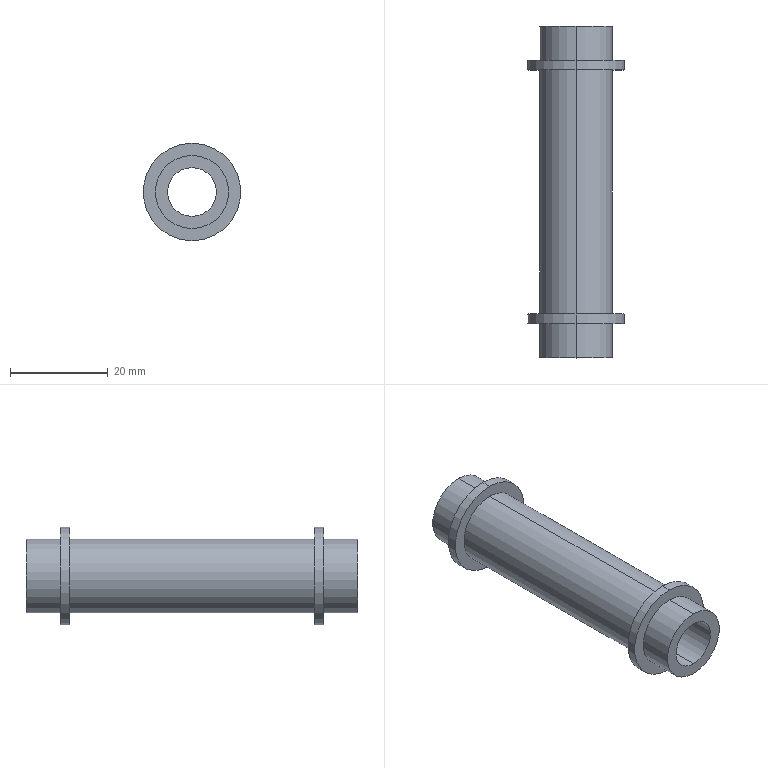Part | STEP file | 1 solid | 18 faces | box 20 x 68 x 20 mm | volume 7226 mm3 | cylinder 12 | plane 6 | commonest cylinder face diameters 15 x6 20 x4 10 x2
STEP:
#1=CARTESIAN_POINT('',(0.,0.,0.));
#2=DIRECTION('',(0.,0.,1.));
#3=DIRECTION('',(1.,0.,0.));
#4=AXIS2_PLACEMENT_3D('',#1,#2,#3);
#5=CARTESIAN_POINT('',(0.,9.,7.5));
#6=VERTEX_POINT('',#5);
#7=CARTESIAN_POINT('',(0.,9.,-7.5));
#8=VERTEX_POINT('',#7);
#9=CARTESIAN_POINT('',(0.,9.,0.));
#10=DIRECTION('',(0.,1.,0.));
#11=DIRECTION('',(0.,0.,1.));
#12=AXIS2_PLACEMENT_3D('',#9,#10,#11);
#13=CIRCLE('',#12,7.5);
#14=CARTESIAN_POINT('',(0.,0.,0.));
#15=DIRECTION('',(0.,1.,0.));
#16=DIRECTION('',(0.,0.,1.));
#17=AXIS2_PLACEMENT_3D('',#14,#15,#16);
#18=CYLINDRICAL_SURFACE('',#17,7.5);
#19=CARTESIAN_POINT('',(0.,9.));
#20=DIRECTION('',(1.,0.));
#21=VECTOR('',#20,1.);
#22=LINE('',#19,#21);
#23=(GEOMETRIC_REPRESENTATION_CONTEXT(2)PARAMETRIC_REPRESENTATION_CONTEXT()REPRESENTATION_CONTEXT('',''));
#24=DEFINITIONAL_REPRESENTATION('',(#22),#23);
#25=PCURVE('',#18,#24);
#26=CARTESIAN_POINT('',(0.,9.,0.));
#27=DIRECTION('',(0.,1.,0.));
#28=DIRECTION('',(0.,0.,1.));
#29=AXIS2_PLACEMENT_3D('',#26,#27,#28);
#30=PLANE('',#29);
#31=CARTESIAN_POINT('',(0.,0.));
#32=DIRECTION('',(1.,0.));
#33=AXIS2_PLACEMENT_2D('',#31,#32);
#34=CIRCLE('',#33,7.5);
#35=(GEOMETRIC_REPRESENTATION_CONTEXT(2)PARAMETRIC_REPRESENTATION_CONTEXT()REPRESENTATION_CONTEXT('',''));
#36=DEFINITIONAL_REPRESENTATION('',(#34),#35);
#37=PCURVE('',#30,#36);
#38=SURFACE_CURVE('',#13,(#25,#37),.PCURVE_S1.);
#39=EDGE_CURVE('',#6,#8,#38,.T.);
#40=ORIENTED_EDGE('',*,*,#39,.T.);
#41=CARTESIAN_POINT('',(0.,59.,-7.5));
#42=VERTEX_POINT('',#41);
#43=CARTESIAN_POINT('',(0.,0.,-7.5));
#44=DIRECTION('',(0.,1.,0.));
#45=VECTOR('',#44,1.);
#46=LINE('',#43,#45);
#47=CARTESIAN_POINT('',(3.142,0.));
#48=DIRECTION('',(0.,1.));
#49=VECTOR('',#48,1.);
#50=LINE('',#47,#49);
#51=(GEOMETRIC_REPRESENTATION_CONTEXT(2)PARAMETRIC_REPRESENTATION_CONTEXT()REPRESENTATION_CONTEXT('',''));
#52=DEFINITIONAL_REPRESENTATION('',(#50),#51);
#53=PCURVE('',#18,#52);
#54=CARTESIAN_POINT('',(0.,0.,0.));
#55=DIRECTION('',(0.,1.,0.));
#56=DIRECTION('',(0.,0.,1.));
#57=AXIS2_PLACEMENT_3D('',#54,#55,#56);
#58=CYLINDRICAL_SURFACE('',#57,7.5);
#59=CARTESIAN_POINT('',(3.142,0.));
#60=DIRECTION('',(0.,1.));
#61=VECTOR('',#60,1.);
#62=LINE('',#59,#61);
#63=(GEOMETRIC_REPRESENTATION_CONTEXT(2)PARAMETRIC_REPRESENTATION_CONTEXT()REPRESENTATION_CONTEXT('',''));
#64=DEFINITIONAL_REPRESENTATION('',(#62),#63);
#65=PCURVE('',#58,#64);
#66=SURFACE_CURVE('',#46,(#53,#65),.PCURVE_S1.);
#67=EDGE_CURVE('',#8,#42,#66,.T.);
#68=ORIENTED_EDGE('',*,*,#67,.T.);
#69=CARTESIAN_POINT('',(0.,59.,7.5));
#70=VERTEX_POINT('',#69);
#71=CARTESIAN_POINT('',(0.,59.,0.));
#72=DIRECTION('',(0.,-1.,0.));
#73=DIRECTION('',(0.,0.,1.));
#74=AXIS2_PLACEMENT_3D('',#71,#72,#73);
#75=CIRCLE('',#74,7.5);
#76=CARTESIAN_POINT('',(6.283,59.));
#77=DIRECTION('',(-1.,0.));
#78=VECTOR('',#77,1.);
#79=LINE('',#76,#78);
#80=(GEOMETRIC_REPRESENTATION_CONTEXT(2)PARAMETRIC_REPRESENTATION_CONTEXT()REPRESENTATION_CONTEXT('',''));
#81=DEFINITIONAL_REPRESENTATION('',(#79),#80);
#82=PCURVE('',#18,#81);
#83=CARTESIAN_POINT('',(0.,59.,0.));
#84=DIRECTION('',(0.,1.,0.));
#85=DIRECTION('',(0.,0.,1.));
#86=AXIS2_PLACEMENT_3D('',#83,#84,#85);
#87=PLANE('',#86);
#88=CARTESIAN_POINT('',(7.5,0.));
#89=CARTESIAN_POINT('',(7.5,-12.99));
#90=CARTESIAN_POINT('',(-3.75,-6.495));
#91=CARTESIAN_POINT('',(-15.,0.));
#92=CARTESIAN_POINT('',(-3.75,6.495));
#93=CARTESIAN_POINT('',(7.5,12.99));
#94=CARTESIAN_POINT('',(7.5,0.));
#95=(BOUNDED_CURVE()B_SPLINE_CURVE(2,(#88,#89,#90,#91,#92,#93,#94),.UNSPECIFIED.,.T.,.F.)B_SPLINE_CURVE_WITH_KNOTS((1,2,2,2,2,1),(-2.094,0.,2.094,4.189,6.283,8.378),.UNSPECIFIED.)CURVE()GEOMETRIC_REPRESENTATION_ITEM()RATIONAL_B_SPLINE_CURVE((1.,0.5,1.,0.5,1.,0.5,1.))REPRESENTATION_ITEM(''));
#96=(GEOMETRIC_REPRESENTATION_CONTEXT(2)PARAMETRIC_REPRESENTATION_CONTEXT()REPRESENTATION_CONTEXT('',''));
#97=DEFINITIONAL_REPRESENTATION('',(#95),#96);
#98=PCURVE('',#87,#97);
#99=SURFACE_CURVE('',#75,(#82,#98),.PCURVE_S1.);
#100=EDGE_CURVE('',#42,#70,#99,.T.);
#101=ORIENTED_EDGE('',*,*,#100,.T.);
#102=CARTESIAN_POINT('',(0.,0.,7.5));
#103=DIRECTION('',(0.,1.,0.));
#104=VECTOR('',#103,1.);
#105=LINE('',#102,#104);
#106=CARTESIAN_POINT('',(0.,0.));
#107=DIRECTION('',(0.,1.));
#108=VECTOR('',#107,1.);
#109=LINE('',#106,#108);
#110=(GEOMETRIC_REPRESENTATION_CONTEXT(2)PARAMETRIC_REPRESENTATION_CONTEXT()REPRESENTATION_CONTEXT('',''));
#111=DEFINITIONAL_REPRESENTATION('',(#109),#110);
#112=PCURVE('',#18,#111);
#113=CARTESIAN_POINT('',(6.283,0.));
#114=DIRECTION('',(0.,1.));
#115=VECTOR('',#114,1.);
#116=LINE('',#113,#115);
#117=(GEOMETRIC_REPRESENTATION_CONTEXT(2)PARAMETRIC_REPRESENTATION_CONTEXT()REPRESENTATION_CONTEXT('',''));
#118=DEFINITIONAL_REPRESENTATION('',(#116),#117);
#119=PCURVE('',#58,#118);
#120=SURFACE_CURVE('',#105,(#112,#119),.PCURVE_S1.);
#121=EDGE_CURVE('',#6,#70,#120,.T.);
#122=ORIENTED_EDGE('',*,*,#121,.F.);
#123=EDGE_LOOP('',(#40,#68,#101,#122));
#124=FACE_BOUND('',#123,.T.);
#125=ADVANCED_FACE('',(#124),#18,.T.);
#126=CARTESIAN_POINT('',(0.,9.,10.));
#127=VERTEX_POINT('',#126);
#128=CARTESIAN_POINT('',(0.,9.,-10.));
#129=VERTEX_POINT('',#128);
#130=CARTESIAN_POINT('',(0.,9.,0.));
#131=DIRECTION('',(0.,1.,0.));
#132=DIRECTION('',(0.,0.,-1.));
#133=AXIS2_PLACEMENT_3D('',#130,#131,#132);
#134=CIRCLE('',#133,10.);
#135=CARTESIAN_POINT('',(0.,9.,0.));
#136=DIRECTION('',(0.,-1.,0.));
#137=DIRECTION('',(0.,0.,-1.));
#138=AXIS2_PLACEMENT_3D('',#135,#136,#137);
#139=CYLINDRICAL_SURFACE('',#138,10.);
#140=CARTESIAN_POINT('',(6.283,0.));
#141=DIRECTION('',(-1.,0.));
#142=VECTOR('',#141,1.);
#143=LINE('',#140,#142);
#144=(GEOMETRIC_REPRESENTATION_CONTEXT(2)PARAMETRIC_REPRESENTATION_CONTEXT()REPRESENTATION_CONTEXT('',''));
#145=DEFINITIONAL_REPRESENTATION('',(#143),#144);
#146=PCURVE('',#139,#145);
#147=CARTESIAN_POINT('',(0.,0.));
#148=DIRECTION('',(-1.,0.));
#149=AXIS2_PLACEMENT_2D('',#147,#148);
#150=CIRCLE('',#149,10.);
#151=(GEOMETRIC_REPRESENTATION_CONTEXT(2)PARAMETRIC_REPRESENTATION_CONTEXT()REPRESENTATION_CONTEXT('',''));
#152=DEFINITIONAL_REPRESENTATION('',(#150),#151);
#153=PCURVE('',#30,#152);
#154=SURFACE_CURVE('',#134,(#146,#153),.PCURVE_S1.);
#155=EDGE_CURVE('',#127,#129,#154,.T.);
#156=ORIENTED_EDGE('',*,*,#155,.F.);
#157=CARTESIAN_POINT('',(0.,7.,10.));
#158=VERTEX_POINT('',#157);
#159=CARTESIAN_POINT('',(0.,9.,10.));
#160=DIRECTION('',(0.,-1.,0.));
#161=VECTOR('',#160,1.);
#162=LINE('',#159,#161);
#163=CARTESIAN_POINT('',(3.142,0.));
#164=DIRECTION('',(0.,1.));
#165=VECTOR('',#164,1.);
#166=LINE('',#163,#165);
#167=(GEOMETRIC_REPRESENTATION_CONTEXT(2)PARAMETRIC_REPRESENTATION_CONTEXT()REPRESENTATION_CONTEXT('',''));
#168=DEFINITIONAL_REPRESENTATION('',(#166),#167);
#169=PCURVE('',#139,#168);
#170=CARTESIAN_POINT('',(0.,9.,0.));
#171=DIRECTION('',(0.,-1.,0.));
#172=DIRECTION('',(0.,0.,-1.));
#173=AXIS2_PLACEMENT_3D('',#170,#171,#172);
#174=CYLINDRICAL_SURFACE('',#173,10.);
#175=CARTESIAN_POINT('',(3.142,0.));
#176=DIRECTION('',(0.,1.));
#177=VECTOR('',#176,1.);
#178=LINE('',#175,#177);
#179=(GEOMETRIC_REPRESENTATION_CONTEXT(2)PARAMETRIC_REPRESENTATION_CONTEXT()REPRESENTATION_CONTEXT('',''));
#180=DEFINITIONAL_REPRESENTATION('',(#178),#179);
#181=PCURVE('',#174,#180);
#182=SURFACE_CURVE('',#162,(#169,#181),.PCURVE_S1.);
#183=EDGE_CURVE('',#127,#158,#182,.T.);
#184=ORIENTED_EDGE('',*,*,#183,.T.);
#185=CARTESIAN_POINT('',(0.,7.,-10.));
#186=VERTEX_POINT('',#185);
#187=CARTESIAN_POINT('',(0.,7.,0.));
#188=DIRECTION('',(0.,1.,0.));
#189=DIRECTION('',(0.,0.,-1.));
#190=AXIS2_PLACEMENT_3D('',#187,#188,#189);
#191=CIRCLE('',#190,10.);
#192=CARTESIAN_POINT('',(6.283,2.));
#193=DIRECTION('',(-1.,0.));
#194=VECTOR('',#193,1.);
#195=LINE('',#192,#194);
#196=(GEOMETRIC_REPRESENTATION_CONTEXT(2)PARAMETRIC_REPRESENTATION_CONTEXT()REPRESENTATION_CONTEXT('',''));
#197=DEFINITIONAL_REPRESENTATION('',(#195),#196);
#198=PCURVE('',#139,#197);
#199=CARTESIAN_POINT('',(0.,7.,0.));
#200=DIRECTION('',(0.,1.,0.));
#201=DIRECTION('',(0.,0.,1.));
#202=AXIS2_PLACEMENT_3D('',#199,#200,#201);
#203=PLANE('',#202);
#204=CARTESIAN_POINT('',(0.,0.));
#205=DIRECTION('',(-1.,0.));
#206=AXIS2_PLACEMENT_2D('',#204,#205);
#207=CIRCLE('',#206,10.);
#208=(GEOMETRIC_REPRESENTATION_CONTEXT(2)PARAMETRIC_REPRESENTATION_CONTEXT()REPRESENTATION_CONTEXT('',''));
#209=DEFINITIONAL_REPRESENTATION('',(#207),#208);
#210=PCURVE('',#203,#209);
#211=SURFACE_CURVE('',#191,(#198,#210),.PCURVE_S1.);
#212=EDGE_CURVE('',#158,#186,#211,.T.);
#213=ORIENTED_EDGE('',*,*,#212,.T.);
#214=CARTESIAN_POINT('',(0.,9.,-10.));
#215=DIRECTION('',(0.,-1.,0.));
#216=VECTOR('',#215,1.);
#217=LINE('',#214,#216);
#218=CARTESIAN_POINT('',(0.,0.));
#219=DIRECTION('',(0.,1.));
#220=VECTOR('',#219,1.);
#221=LINE('',#218,#220);
#222=(GEOMETRIC_REPRESENTATION_CONTEXT(2)PARAMETRIC_REPRESENTATION_CONTEXT()REPRESENTATION_CONTEXT('',''));
#223=DEFINITIONAL_REPRESENTATION('',(#221),#222);
#224=PCURVE('',#139,#223);
#225=CARTESIAN_POINT('',(6.283,0.));
#226=DIRECTION('',(0.,1.));
#227=VECTOR('',#226,1.);
#228=LINE('',#225,#227);
#229=(GEOMETRIC_REPRESENTATION_CONTEXT(2)PARAMETRIC_REPRESENTATION_CONTEXT()REPRESENTATION_CONTEXT('',''));
#230=DEFINITIONAL_REPRESENTATION('',(#228),#229);
#231=PCURVE('',#174,#230);
#232=SURFACE_CURVE('',#217,(#224,#231),.PCURVE_S1.);
#233=EDGE_CURVE('',#129,#186,#232,.T.);
#234=ORIENTED_EDGE('',*,*,#233,.F.);
#235=EDGE_LOOP('',(#156,#184,#213,#234));
#236=FACE_BOUND('',#235,.T.);
#237=ADVANCED_FACE('',(#236),#139,.T.);
#238=CARTESIAN_POINT('',(0.,61.,-10.));
#239=VERTEX_POINT('',#238);
#240=CARTESIAN_POINT('',(0.,61.,10.));
#241=VERTEX_POINT('',#240);
#242=CARTESIAN_POINT('',(0.,61.,0.));
#243=DIRECTION('',(0.,-1.,0.));
#244=DIRECTION('',(0.,0.,-1.));
#245=AXIS2_PLACEMENT_3D('',#242,#243,#244);
#246=CIRCLE('',#245,10.);
#247=CARTESIAN_POINT('',(0.,59.,0.));
#248=DIRECTION('',(0.,-1.,0.));
#249=DIRECTION('',(0.,0.,-1.));
#250=AXIS2_PLACEMENT_3D('',#247,#248,#249);
#251=CYLINDRICAL_SURFACE('',#250,10.);
#252=CARTESIAN_POINT('',(0.,-2.));
#253=DIRECTION('',(1.,0.));
#254=VECTOR('',#253,1.);
#255=LINE('',#252,#254);
#256=(GEOMETRIC_REPRESENTATION_CONTEXT(2)PARAMETRIC_REPRESENTATION_CONTEXT()REPRESENTATION_CONTEXT('',''));
#257=DEFINITIONAL_REPRESENTATION('',(#255),#256);
#258=PCURVE('',#251,#257);
#259=CARTESIAN_POINT('',(0.,61.,0.));
#260=DIRECTION('',(0.,1.,0.));
#261=DIRECTION('',(0.,0.,1.));
#262=AXIS2_PLACEMENT_3D('',#259,#260,#261);
#263=PLANE('',#262);
#264=CARTESIAN_POINT('',(-10.,0.));
#265=CARTESIAN_POINT('',(-10.,17.321));
#266=CARTESIAN_POINT('',(5.,8.66));
#267=CARTESIAN_POINT('',(20.,0.));
#268=CARTESIAN_POINT('',(5.,-8.66));
#269=CARTESIAN_POINT('',(-10.,-17.321));
#270=CARTESIAN_POINT('',(-10.,0.));
#271=(BOUNDED_CURVE()B_SPLINE_CURVE(2,(#264,#265,#266,#267,#268,#269,#270),.UNSPECIFIED.,.T.,.F.)B_SPLINE_CURVE_WITH_KNOTS((1,2,2,2,2,1),(-2.094,0.,2.094,4.189,6.283,8.378),.UNSPECIFIED.)CURVE()GEOMETRIC_REPRESENTATION_ITEM()RATIONAL_B_SPLINE_CURVE((1.,0.5,1.,0.5,1.,0.5,1.))REPRESENTATION_ITEM(''));
#272=(GEOMETRIC_REPRESENTATION_CONTEXT(2)PARAMETRIC_REPRESENTATION_CONTEXT()REPRESENTATION_CONTEXT('',''));
#273=DEFINITIONAL_REPRESENTATION('',(#271),#272);
#274=PCURVE('',#263,#273);
#275=SURFACE_CURVE('',#246,(#258,#274),.PCURVE_S1.);
#276=EDGE_CURVE('',#239,#241,#275,.T.);
#277=ORIENTED_EDGE('',*,*,#276,.T.);
#278=CARTESIAN_POINT('',(0.,59.,10.));
#279=VERTEX_POINT('',#278);
#280=CARTESIAN_POINT('',(0.,59.,10.));
#281=DIRECTION('',(0.,-1.,0.));
#282=VECTOR('',#281,1.);
#283=LINE('',#280,#282);
#284=CARTESIAN_POINT('',(3.142,0.));
#285=DIRECTION('',(0.,1.));
#286=VECTOR('',#285,1.);
#287=LINE('',#284,#286);
#288=(GEOMETRIC_REPRESENTATION_CONTEXT(2)PARAMETRIC_REPRESENTATION_CONTEXT()REPRESENTATION_CONTEXT('',''));
#289=DEFINITIONAL_REPRESENTATION('',(#287),#288);
#290=PCURVE('',#251,#289);
#291=CARTESIAN_POINT('',(0.,59.,0.));
#292=DIRECTION('',(0.,-1.,0.));
#293=DIRECTION('',(0.,0.,-1.));
#294=AXIS2_PLACEMENT_3D('',#291,#292,#293);
#295=CYLINDRICAL_SURFACE('',#294,10.);
#296=CARTESIAN_POINT('',(3.142,0.));
#297=DIRECTION('',(0.,1.));
#298=VECTOR('',#297,1.);
#299=LINE('',#296,#298);
#300=(GEOMETRIC_REPRESENTATION_CONTEXT(2)PARAMETRIC_REPRESENTATION_CONTEXT()REPRESENTATION_CONTEXT('',''));
#301=DEFINITIONAL_REPRESENTATION('',(#299),#300);
#302=PCURVE('',#295,#301);
#303=SURFACE_CURVE('',#283,(#290,#302),.PCURVE_S1.);
#304=EDGE_CURVE('',#241,#279,#303,.T.);
#305=ORIENTED_EDGE('',*,*,#304,.T.);
#306=CARTESIAN_POINT('',(0.,59.,-10.));
#307=VERTEX_POINT('',#306);
#308=CARTESIAN_POINT('',(0.,59.,0.));
#309=DIRECTION('',(0.,1.,0.));
#310=DIRECTION('',(0.,0.,-1.));
#311=AXIS2_PLACEMENT_3D('',#308,#309,#310);
#312=CIRCLE('',#311,10.);
#313=CARTESIAN_POINT('',(6.283,0.));
#314=DIRECTION('',(-1.,0.));
#315=VECTOR('',#314,1.);
#316=LINE('',#313,#315);
#317=(GEOMETRIC_REPRESENTATION_CONTEXT(2)PARAMETRIC_REPRESENTATION_CONTEXT()REPRESENTATION_CONTEXT('',''));
#318=DEFINITIONAL_REPRESENTATION('',(#316),#317);
#319=PCURVE('',#251,#318);
#320=CARTESIAN_POINT('',(0.,0.));
#321=DIRECTION('',(-1.,0.));
#322=AXIS2_PLACEMENT_2D('',#320,#321);
#323=CIRCLE('',#322,10.);
#324=(GEOMETRIC_REPRESENTATION_CONTEXT(2)PARAMETRIC_REPRESENTATION_CONTEXT()REPRESENTATION_CONTEXT('',''));
#325=DEFINITIONAL_REPRESENTATION('',(#323),#324);
#326=PCURVE('',#87,#325);
#327=SURFACE_CURVE('',#312,(#319,#326),.PCURVE_S1.);
#328=EDGE_CURVE('',#279,#307,#327,.T.);
#329=ORIENTED_EDGE('',*,*,#328,.T.);
#330=CARTESIAN_POINT('',(0.,59.,-10.));
#331=DIRECTION('',(0.,-1.,0.));
#332=VECTOR('',#331,1.);
#333=LINE('',#330,#332);
#334=CARTESIAN_POINT('',(0.,0.));
#335=DIRECTION('',(0.,1.));
#336=VECTOR('',#335,1.);
#337=LINE('',#334,#336);
#338=(GEOMETRIC_REPRESENTATION_CONTEXT(2)PARAMETRIC_REPRESENTATION_CONTEXT()REPRESENTATION_CONTEXT('',''));
#339=DEFINITIONAL_REPRESENTATION('',(#337),#338);
#340=PCURVE('',#251,#339);
#341=CARTESIAN_POINT('',(6.283,0.));
#342=DIRECTION('',(0.,1.));
#343=VECTOR('',#342,1.);
#344=LINE('',#341,#343);
#345=(GEOMETRIC_REPRESENTATION_CONTEXT(2)PARAMETRIC_REPRESENTATION_CONTEXT()REPRESENTATION_CONTEXT('',''));
#346=DEFINITIONAL_REPRESENTATION('',(#344),#345);
#347=PCURVE('',#295,#346);
#348=SURFACE_CURVE('',#333,(#340,#347),.PCURVE_S1.);
#349=EDGE_CURVE('',#239,#307,#348,.T.);
#350=ORIENTED_EDGE('',*,*,#349,.F.);
#351=EDGE_LOOP('',(#277,#305,#329,#350));
#352=FACE_BOUND('',#351,.T.);
#353=ADVANCED_FACE('',(#352),#251,.T.);
#354=CARTESIAN_POINT('',(0.,0.,7.5));
#355=VERTEX_POINT('',#354);
#356=CARTESIAN_POINT('',(0.,0.,-7.5));
#357=VERTEX_POINT('',#356);
#358=CARTESIAN_POINT('',(0.,0.,0.));
#359=DIRECTION('',(0.,1.,0.));
#360=DIRECTION('',(0.,0.,1.));
#361=AXIS2_PLACEMENT_3D('',#358,#359,#360);
#362=CIRCLE('',#361,7.5);
#363=CARTESIAN_POINT('',(0.,0.,0.));
#364=DIRECTION('',(0.,1.,0.));
#365=DIRECTION('',(0.,0.,1.));
#366=AXIS2_PLACEMENT_3D('',#363,#364,#365);
#367=CYLINDRICAL_SURFACE('',#366,7.5);
#368=CARTESIAN_POINT('',(0.,0.));
#369=DIRECTION('',(1.,0.));
#370=VECTOR('',#369,1.);
#371=LINE('',#368,#370);
#372=(GEOMETRIC_REPRESENTATION_CONTEXT(2)PARAMETRIC_REPRESENTATION_CONTEXT()REPRESENTATION_CONTEXT('',''));
#373=DEFINITIONAL_REPRESENTATION('',(#371),#372);
#374=PCURVE('',#367,#373);
#375=CARTESIAN_POINT('',(0.,0.,0.));
#376=DIRECTION('',(0.,1.,0.));
#377=DIRECTION('',(0.,0.,1.));
#378=AXIS2_PLACEMENT_3D('',#375,#376,#377);
#379=PLANE('',#378);
#380=CARTESIAN_POINT('',(0.,0.));
#381=DIRECTION('',(1.,0.));
#382=AXIS2_PLACEMENT_2D('',#380,#381);
#383=CIRCLE('',#382,7.5);
#384=(GEOMETRIC_REPRESENTATION_CONTEXT(2)PARAMETRIC_REPRESENTATION_CONTEXT()REPRESENTATION_CONTEXT('',''));
#385=DEFINITIONAL_REPRESENTATION('',(#383),#384);
#386=PCURVE('',#379,#385);
#387=SURFACE_CURVE('',#362,(#374,#386),.PCURVE_S1.);
#388=EDGE_CURVE('',#355,#357,#387,.T.);
#389=ORIENTED_EDGE('',*,*,#388,.T.);
#390=CARTESIAN_POINT('',(0.,7.,-7.5));
#391=VERTEX_POINT('',#390);
#392=CARTESIAN_POINT('',(0.,0.,-7.5));
#393=DIRECTION('',(0.,1.,0.));
#394=VECTOR('',#393,1.);
#395=LINE('',#392,#394);
#396=CARTESIAN_POINT('',(3.142,0.));
#397=DIRECTION('',(0.,1.));
#398=VECTOR('',#397,1.);
#399=LINE('',#396,#398);
#400=(GEOMETRIC_REPRESENTATION_CONTEXT(2)PARAMETRIC_REPRESENTATION_CONTEXT()REPRESENTATION_CONTEXT('',''));
#401=DEFINITIONAL_REPRESENTATION('',(#399),#400);
#402=PCURVE('',#367,#401);
#403=CARTESIAN_POINT('',(0.,0.,0.));
#404=DIRECTION('',(0.,1.,0.));
#405=DIRECTION('',(0.,0.,1.));
#406=AXIS2_PLACEMENT_3D('',#403,#404,#405);
#407=CYLINDRICAL_SURFACE('',#406,7.5);
#408=CARTESIAN_POINT('',(3.142,0.));
#409=DIRECTION('',(0.,1.));
#410=VECTOR('',#409,1.);
#411=LINE('',#408,#410);
#412=(GEOMETRIC_REPRESENTATION_CONTEXT(2)PARAMETRIC_REPRESENTATION_CONTEXT()REPRESENTATION_CONTEXT('',''));
#413=DEFINITIONAL_REPRESENTATION('',(#411),#412);
#414=PCURVE('',#407,#413);
#415=SURFACE_CURVE('',#395,(#402,#414),.PCURVE_S1.);
#416=EDGE_CURVE('',#357,#391,#415,.T.);
#417=ORIENTED_EDGE('',*,*,#416,.T.);
#418=CARTESIAN_POINT('',(0.,7.,7.5));
#419=VERTEX_POINT('',#418);
#420=CARTESIAN_POINT('',(0.,7.,0.));
#421=DIRECTION('',(0.,-1.,0.));
#422=DIRECTION('',(0.,0.,1.));
#423=AXIS2_PLACEMENT_3D('',#420,#421,#422);
#424=CIRCLE('',#423,7.5);
#425=CARTESIAN_POINT('',(6.283,7.));
#426=DIRECTION('',(-1.,0.));
#427=VECTOR('',#426,1.);
#428=LINE('',#425,#427);
#429=(GEOMETRIC_REPRESENTATION_CONTEXT(2)PARAMETRIC_REPRESENTATION_CONTEXT()REPRESENTATION_CONTEXT('',''));
#430=DEFINITIONAL_REPRESENTATION('',(#428),#429);
#431=PCURVE('',#367,#430);
#432=CARTESIAN_POINT('',(7.5,0.));
#433=CARTESIAN_POINT('',(7.5,-12.99));
#434=CARTESIAN_POINT('',(-3.75,-6.495));
#435=CARTESIAN_POINT('',(-15.,0.));
#436=CARTESIAN_POINT('',(-3.75,6.495));
#437=CARTESIAN_POINT('',(7.5,12.99));
#438=CARTESIAN_POINT('',(7.5,0.));
#439=(BOUNDED_CURVE()B_SPLINE_CURVE(2,(#432,#433,#434,#435,#436,#437,#438),.UNSPECIFIED.,.T.,.F.)B_SPLINE_CURVE_WITH_KNOTS((1,2,2,2,2,1),(-2.094,0.,2.094,4.189,6.283,8.378),.UNSPECIFIED.)CURVE()GEOMETRIC_REPRESENTATION_ITEM()RATIONAL_B_SPLINE_CURVE((1.,0.5,1.,0.5,1.,0.5,1.))REPRESENTATION_ITEM(''));
#440=(GEOMETRIC_REPRESENTATION_CONTEXT(2)PARAMETRIC_REPRESENTATION_CONTEXT()REPRESENTATION_CONTEXT('',''));
#441=DEFINITIONAL_REPRESENTATION('',(#439),#440);
#442=PCURVE('',#203,#441);
#443=SURFACE_CURVE('',#424,(#431,#442),.PCURVE_S1.);
#444=EDGE_CURVE('',#391,#419,#443,.T.);
#445=ORIENTED_EDGE('',*,*,#444,.T.);
#446=CARTESIAN_POINT('',(0.,0.,7.5));
#447=DIRECTION('',(0.,1.,0.));
#448=VECTOR('',#447,1.);
#449=LINE('',#446,#448);
#450=CARTESIAN_POINT('',(0.,0.));
#451=DIRECTION('',(0.,1.));
#452=VECTOR('',#451,1.);
#453=LINE('',#450,#452);
#454=(GEOMETRIC_REPRESENTATION_CONTEXT(2)PARAMETRIC_REPRESENTATION_CONTEXT()REPRESENTATION_CONTEXT('',''));
#455=DEFINITIONAL_REPRESENTATION('',(#453),#454);
#456=PCURVE('',#367,#455);
#457=CARTESIAN_POINT('',(6.283,0.));
#458=DIRECTION('',(0.,1.));
#459=VECTOR('',#458,1.);
#460=LINE('',#457,#459);
#461=(GEOMETRIC_REPRESENTATION_CONTEXT(2)PARAMETRIC_REPRESENTATION_CONTEXT()REPRESENTATION_CONTEXT('',''));
#462=DEFINITIONAL_REPRESENTATION('',(#460),#461);
#463=PCURVE('',#407,#462);
#464=SURFACE_CURVE('',#449,(#456,#463),.PCURVE_S1.);
#465=EDGE_CURVE('',#355,#419,#464,.T.);
#466=ORIENTED_EDGE('',*,*,#465,.F.);
#467=EDGE_LOOP('',(#389,#417,#445,#466));
#468=FACE_BOUND('',#467,.T.);
#469=ADVANCED_FACE('',(#468),#367,.T.);
#470=CARTESIAN_POINT('',(0.,61.,-7.5));
#471=VERTEX_POINT('',#470);
#472=CARTESIAN_POINT('',(0.,61.,7.5));
#473=VERTEX_POINT('',#472);
#474=CARTESIAN_POINT('',(0.,61.,0.));
#475=DIRECTION('',(0.,-1.,0.));
#476=DIRECTION('',(0.,0.,1.));
#477=AXIS2_PLACEMENT_3D('',#474,#475,#476);
#478=CIRCLE('',#477,7.5);
#479=CARTESIAN_POINT('',(0.,0.,0.));
#480=DIRECTION('',(0.,1.,0.));
#481=DIRECTION('',(0.,0.,1.));
#482=AXIS2_PLACEMENT_3D('',#479,#480,#481);
#483=CYLINDRICAL_SURFACE('',#482,7.5);
#484=CARTESIAN_POINT('',(6.283,61.));
#485=DIRECTION('',(-1.,0.));
#486=VECTOR('',#485,1.);
#487=LINE('',#484,#486);
#488=(GEOMETRIC_REPRESENTATION_CONTEXT(2)PARAMETRIC_REPRESENTATION_CONTEXT()REPRESENTATION_CONTEXT('',''));
#489=DEFINITIONAL_REPRESENTATION('',(#487),#488);
#490=PCURVE('',#483,#489);
#491=CARTESIAN_POINT('',(7.5,0.));
#492=CARTESIAN_POINT('',(7.5,-12.99));
#493=CARTESIAN_POINT('',(-3.75,-6.495));
#494=CARTESIAN_POINT('',(-15.,0.));
#495=CARTESIAN_POINT('',(-3.75,6.495));
#496=CARTESIAN_POINT('',(7.5,12.99));
#497=CARTESIAN_POINT('',(7.5,0.));
#498=(BOUNDED_CURVE()B_SPLINE_CURVE(2,(#491,#492,#493,#494,#495,#496,#497),.UNSPECIFIED.,.T.,.F.)B_SPLINE_CURVE_WITH_KNOTS((1,2,2,2,2,1),(-2.094,0.,2.094,4.189,6.283,8.378),.UNSPECIFIED.)CURVE()GEOMETRIC_REPRESENTATION_ITEM()RATIONAL_B_SPLINE_CURVE((1.,0.5,1.,0.5,1.,0.5,1.))REPRESENTATION_ITEM(''));
#499=(GEOMETRIC_REPRESENTATION_CONTEXT(2)PARAMETRIC_REPRESENTATION_CONTEXT()REPRESENTATION_CONTEXT('',''));
#500=DEFINITIONAL_REPRESENTATION('',(#498),#499);
#501=PCURVE('',#263,#500);
#502=SURFACE_CURVE('',#478,(#490,#501),.PCURVE_S1.);
#503=EDGE_CURVE('',#471,#473,#502,.T.);
#504=ORIENTED_EDGE('',*,*,#503,.F.);
#505=CARTESIAN_POINT('',(0.,68.,-7.5));
#506=VERTEX_POINT('',#505);
#507=CARTESIAN_POINT('',(0.,0.,-7.5));
#508=DIRECTION('',(0.,1.,0.));
#509=VECTOR('',#508,1.);
#510=LINE('',#507,#509);
#511=CARTESIAN_POINT('',(3.142,0.));
#512=DIRECTION('',(0.,1.));
#513=VECTOR('',#512,1.);
#514=LINE('',#511,#513);
#515=(GEOMETRIC_REPRESENTATION_CONTEXT(2)PARAMETRIC_REPRESENTATION_CONTEXT()REPRESENTATION_CONTEXT('',''));
#516=DEFINITIONAL_REPRESENTATION('',(#514),#515);
#517=PCURVE('',#483,#516);
#518=CARTESIAN_POINT('',(0.,0.,0.));
#519=DIRECTION('',(0.,1.,0.));
#520=DIRECTION('',(0.,0.,1.));
#521=AXIS2_PLACEMENT_3D('',#518,#519,#520);
#522=CYLINDRICAL_SURFACE('',#521,7.5);
#523=CARTESIAN_POINT('',(3.142,0.));
#524=DIRECTION('',(0.,1.));
#525=VECTOR('',#524,1.);
#526=LINE('',#523,#525);
#527=(GEOMETRIC_REPRESENTATION_CONTEXT(2)PARAMETRIC_REPRESENTATION_CONTEXT()REPRESENTATION_CONTEXT('',''));
#528=DEFINITIONAL_REPRESENTATION('',(#526),#527);
#529=PCURVE('',#522,#528);
#530=SURFACE_CURVE('',#510,(#517,#529),.PCURVE_S1.);
#531=EDGE_CURVE('',#471,#506,#530,.T.);
#532=ORIENTED_EDGE('',*,*,#531,.T.);
#533=CARTESIAN_POINT('',(0.,68.,7.5));
#534=VERTEX_POINT('',#533);
#535=CARTESIAN_POINT('',(0.,68.,0.));
#536=DIRECTION('',(0.,-1.,0.));
#537=DIRECTION('',(0.,0.,1.));
#538=AXIS2_PLACEMENT_3D('',#535,#536,#537);
#539=CIRCLE('',#538,7.5);
#540=CARTESIAN_POINT('',(6.283,68.));
#541=DIRECTION('',(-1.,0.));
#542=VECTOR('',#541,1.);
#543=LINE('',#540,#542);
#544=(GEOMETRIC_REPRESENTATION_CONTEXT(2)PARAMETRIC_REPRESENTATION_CONTEXT()REPRESENTATION_CONTEXT('',''));
#545=DEFINITIONAL_REPRESENTATION('',(#543),#544);
#546=PCURVE('',#483,#545);
#547=CARTESIAN_POINT('',(0.,68.,0.));
#548=DIRECTION('',(0.,1.,0.));
#549=DIRECTION('',(0.,0.,1.));
#550=AXIS2_PLACEMENT_3D('',#547,#548,#549);
#551=PLANE('',#550);
#552=CARTESIAN_POINT('',(7.5,0.));
#553=CARTESIAN_POINT('',(7.5,-12.99));
#554=CARTESIAN_POINT('',(-3.75,-6.495));
#555=CARTESIAN_POINT('',(-15.,0.));
#556=CARTESIAN_POINT('',(-3.75,6.495));
#557=CARTESIAN_POINT('',(7.5,12.99));
#558=CARTESIAN_POINT('',(7.5,0.));
#559=(BOUNDED_CURVE()B_SPLINE_CURVE(2,(#552,#553,#554,#555,#556,#557,#558),.UNSPECIFIED.,.T.,.F.)B_SPLINE_CURVE_WITH_KNOTS((1,2,2,2,2,1),(-2.094,0.,2.094,4.189,6.283,8.378),.UNSPECIFIED.)CURVE()GEOMETRIC_REPRESENTATION_ITEM()RATIONAL_B_SPLINE_CURVE((1.,0.5,1.,0.5,1.,0.5,1.))REPRESENTATION_ITEM(''));
#560=(GEOMETRIC_REPRESENTATION_CONTEXT(2)PARAMETRIC_REPRESENTATION_CONTEXT()REPRESENTATION_CONTEXT('',''));
#561=DEFINITIONAL_REPRESENTATION('',(#559),#560);
#562=PCURVE('',#551,#561);
#563=SURFACE_CURVE('',#539,(#546,#562),.PCURVE_S1.);
#564=EDGE_CURVE('',#506,#534,#563,.T.);
#565=ORIENTED_EDGE('',*,*,#564,.T.);
#566=CARTESIAN_POINT('',(0.,0.,7.5));
#567=DIRECTION('',(0.,1.,0.));
#568=VECTOR('',#567,1.);
#569=LINE('',#566,#568);
#570=CARTESIAN_POINT('',(0.,0.));
#571=DIRECTION('',(0.,1.));
#572=VECTOR('',#571,1.);
#573=LINE('',#570,#572);
#574=(GEOMETRIC_REPRESENTATION_CONTEXT(2)PARAMETRIC_REPRESENTATION_CONTEXT()REPRESENTATION_CONTEXT('',''));
#575=DEFINITIONAL_REPRESENTATION('',(#573),#574);
#576=PCURVE('',#483,#575);
#577=CARTESIAN_POINT('',(6.283,0.));
#578=DIRECTION('',(0.,1.));
#579=VECTOR('',#578,1.);
#580=LINE('',#577,#579);
#581=(GEOMETRIC_REPRESENTATION_CONTEXT(2)PARAMETRIC_REPRESENTATION_CONTEXT()REPRESENTATION_CONTEXT('',''));
#582=DEFINITIONAL_REPRESENTATION('',(#580),#581);
#583=PCURVE('',#522,#582);
#584=SURFACE_CURVE('',#569,(#576,#583),.PCURVE_S1.);
#585=EDGE_CURVE('',#473,#534,#584,.T.);
#586=ORIENTED_EDGE('',*,*,#585,.F.);
#587=EDGE_LOOP('',(#504,#532,#565,#586));
#588=FACE_BOUND('',#587,.T.);
#589=ADVANCED_FACE('',(#588),#483,.T.);
#590=CARTESIAN_POINT('',(0.,0.,5.));
#591=VERTEX_POINT('',#590);
#592=CARTESIAN_POINT('',(0.,68.,5.));
#593=VERTEX_POINT('',#592);
#594=CARTESIAN_POINT('',(0.,0.,5.));
#595=DIRECTION('',(0.,1.,0.));
#596=VECTOR('',#595,1.);
#597=LINE('',#594,#596);
#598=CARTESIAN_POINT('',(0.,0.,0.));
#599=DIRECTION('',(0.,1.,0.));
#600=DIRECTION('',(0.,0.,1.));
#601=AXIS2_PLACEMENT_3D('',#598,#599,#600);
#602=CYLINDRICAL_SURFACE('',#601,5.);
#603=CARTESIAN_POINT('',(6.283,0.));
#604=DIRECTION('',(0.,1.));
#605=VECTOR('',#604,1.);
#606=LINE('',#603,#605);
#607=(GEOMETRIC_REPRESENTATION_CONTEXT(2)PARAMETRIC_REPRESENTATION_CONTEXT()REPRESENTATION_CONTEXT('',''));
#608=DEFINITIONAL_REPRESENTATION('',(#606),#607);
#609=PCURVE('',#602,#608);
#610=CARTESIAN_POINT('',(0.,0.,0.));
#611=DIRECTION('',(0.,1.,0.));
#612=DIRECTION('',(0.,0.,1.));
#613=AXIS2_PLACEMENT_3D('',#610,#611,#612);
#614=CYLINDRICAL_SURFACE('',#613,5.);
#615=CARTESIAN_POINT('',(0.,0.));
#616=DIRECTION('',(0.,1.));
#617=VECTOR('',#616,1.);
#618=LINE('',#615,#617);
#619=(GEOMETRIC_REPRESENTATION_CONTEXT(2)PARAMETRIC_REPRESENTATION_CONTEXT()REPRESENTATION_CONTEXT('',''));
#620=DEFINITIONAL_REPRESENTATION('',(#618),#619);
#621=PCURVE('',#614,#620);
#622=SURFACE_CURVE('',#597,(#609,#621),.PCURVE_S1.);
#623=EDGE_CURVE('',#591,#593,#622,.T.);
#624=ORIENTED_EDGE('',*,*,#623,.T.);
#625=CARTESIAN_POINT('',(0.,68.,-5.));
#626=VERTEX_POINT('',#625);
#627=CARTESIAN_POINT('',(0.,68.,0.));
#628=DIRECTION('',(0.,-1.,0.));
#629=DIRECTION('',(0.,0.,1.));
#630=AXIS2_PLACEMENT_3D('',#627,#628,#629);
#631=CIRCLE('',#630,5.);
#632=CARTESIAN_POINT('',(6.283,68.));
#633=DIRECTION('',(-1.,0.));
#634=VECTOR('',#633,1.);
#635=LINE('',#632,#634);
#636=(GEOMETRIC_REPRESENTATION_CONTEXT(2)PARAMETRIC_REPRESENTATION_CONTEXT()REPRESENTATION_CONTEXT('',''));
#637=DEFINITIONAL_REPRESENTATION('',(#635),#636);
#638=PCURVE('',#602,#637);
#639=CARTESIAN_POINT('',(5.,0.));
#640=CARTESIAN_POINT('',(5.,-8.66));
#641=CARTESIAN_POINT('',(-2.5,-4.33));
#642=CARTESIAN_POINT('',(-10.,0.));
#643=CARTESIAN_POINT('',(-2.5,4.33));
#644=CARTESIAN_POINT('',(5.,8.66));
#645=CARTESIAN_POINT('',(5.,0.));
#646=(BOUNDED_CURVE()B_SPLINE_CURVE(2,(#639,#640,#641,#642,#643,#644,#645),.UNSPECIFIED.,.T.,.F.)B_SPLINE_CURVE_WITH_KNOTS((1,2,2,2,2,1),(-2.094,0.,2.094,4.189,6.283,8.378),.UNSPECIFIED.)CURVE()GEOMETRIC_REPRESENTATION_ITEM()RATIONAL_B_SPLINE_CURVE((1.,0.5,1.,0.5,1.,0.5,1.))REPRESENTATION_ITEM(''));
#647=(GEOMETRIC_REPRESENTATION_CONTEXT(2)PARAMETRIC_REPRESENTATION_CONTEXT()REPRESENTATION_CONTEXT('',''));
#648=DEFINITIONAL_REPRESENTATION('',(#646),#647);
#649=PCURVE('',#551,#648);
#650=SURFACE_CURVE('',#631,(#638,#649),.PCURVE_S1.);
#651=EDGE_CURVE('',#593,#626,#650,.T.);
#652=ORIENTED_EDGE('',*,*,#651,.T.);
#653=CARTESIAN_POINT('',(0.,0.,-5.));
#654=VERTEX_POINT('',#653);
#655=CARTESIAN_POINT('',(0.,0.,-5.));
#656=DIRECTION('',(0.,1.,0.));
#657=VECTOR('',#656,1.);
#658=LINE('',#655,#657);
#659=CARTESIAN_POINT('',(3.142,0.));
#660=DIRECTION('',(0.,1.));
#661=VECTOR('',#660,1.);
#662=LINE('',#659,#661);
#663=(GEOMETRIC_REPRESENTATION_CONTEXT(2)PARAMETRIC_REPRESENTATION_CONTEXT()REPRESENTATION_CONTEXT('',''));
#664=DEFINITIONAL_REPRESENTATION('',(#662),#663);
#665=PCURVE('',#602,#664);
#666=CARTESIAN_POINT('',(3.142,0.));
#667=DIRECTION('',(0.,1.));
#668=VECTOR('',#667,1.);
#669=LINE('',#666,#668);
#670=(GEOMETRIC_REPRESENTATION_CONTEXT(2)PARAMETRIC_REPRESENTATION_CONTEXT()REPRESENTATION_CONTEXT('',''));
#671=DEFINITIONAL_REPRESENTATION('',(#669),#670);
#672=PCURVE('',#614,#671);
#673=SURFACE_CURVE('',#658,(#665,#672),.PCURVE_S1.);
#674=EDGE_CURVE('',#654,#626,#673,.T.);
#675=ORIENTED_EDGE('',*,*,#674,.F.);
#676=CARTESIAN_POINT('',(0.,0.,0.));
#677=DIRECTION('',(0.,-1.,0.));
#678=DIRECTION('',(0.,0.,1.));
#679=AXIS2_PLACEMENT_3D('',#676,#677,#678);
#680=CIRCLE('',#679,5.);
#681=CARTESIAN_POINT('',(6.283,0.));
#682=DIRECTION('',(-1.,0.));
#683=VECTOR('',#682,1.);
#684=LINE('',#681,#683);
#685=(GEOMETRIC_REPRESENTATION_CONTEXT(2)PARAMETRIC_REPRESENTATION_CONTEXT()REPRESENTATION_CONTEXT('',''));
#686=DEFINITIONAL_REPRESENTATION('',(#684),#685);
#687=PCURVE('',#602,#686);
#688=CARTESIAN_POINT('',(5.,0.));
#689=CARTESIAN_POINT('',(5.,-8.66));
#690=CARTESIAN_POINT('',(-2.5,-4.33));
#691=CARTESIAN_POINT('',(-10.,0.));
#692=CARTESIAN_POINT('',(-2.5,4.33));
#693=CARTESIAN_POINT('',(5.,8.66));
#694=CARTESIAN_POINT('',(5.,0.));
#695=(BOUNDED_CURVE()B_SPLINE_CURVE(2,(#688,#689,#690,#691,#692,#693,#694),.UNSPECIFIED.,.T.,.F.)B_SPLINE_CURVE_WITH_KNOTS((1,2,2,2,2,1),(-2.094,0.,2.094,4.189,6.283,8.378),.UNSPECIFIED.)CURVE()GEOMETRIC_REPRESENTATION_ITEM()RATIONAL_B_SPLINE_CURVE((1.,0.5,1.,0.5,1.,0.5,1.))REPRESENTATION_ITEM(''));
#696=(GEOMETRIC_REPRESENTATION_CONTEXT(2)PARAMETRIC_REPRESENTATION_CONTEXT()REPRESENTATION_CONTEXT('',''));
#697=DEFINITIONAL_REPRESENTATION('',(#695),#696);
#698=PCURVE('',#379,#697);
#699=SURFACE_CURVE('',#680,(#687,#698),.PCURVE_S1.);
#700=EDGE_CURVE('',#591,#654,#699,.T.);
#701=ORIENTED_EDGE('',*,*,#700,.F.);
#702=EDGE_LOOP('',(#624,#652,#675,#701));
#703=FACE_BOUND('',#702,.F.);
#704=ADVANCED_FACE('',(#703),#602,.F.);
#705=ORIENTED_EDGE('',*,*,#67,.F.);
#706=CARTESIAN_POINT('',(0.,9.,0.));
#707=DIRECTION('',(0.,1.,0.));
#708=DIRECTION('',(0.,0.,1.));
#709=AXIS2_PLACEMENT_3D('',#706,#707,#708);
#710=CIRCLE('',#709,7.5);
#711=CARTESIAN_POINT('',(0.,9.));
#712=DIRECTION('',(1.,0.));
#713=VECTOR('',#712,1.);
#714=LINE('',#711,#713);
#715=(GEOMETRIC_REPRESENTATION_CONTEXT(2)PARAMETRIC_REPRESENTATION_CONTEXT()REPRESENTATION_CONTEXT('',''));
#716=DEFINITIONAL_REPRESENTATION('',(#714),#715);
#717=PCURVE('',#58,#716);
#718=CARTESIAN_POINT('',(0.,0.));
#719=DIRECTION('',(1.,0.));
#720=AXIS2_PLACEMENT_2D('',#718,#719);
#721=CIRCLE('',#720,7.5);
#722=(GEOMETRIC_REPRESENTATION_CONTEXT(2)PARAMETRIC_REPRESENTATION_CONTEXT()REPRESENTATION_CONTEXT('',''));
#723=DEFINITIONAL_REPRESENTATION('',(#721),#722);
#724=PCURVE('',#30,#723);
#725=SURFACE_CURVE('',#710,(#717,#724),.PCURVE_S1.);
#726=EDGE_CURVE('',#8,#6,#725,.T.);
#727=ORIENTED_EDGE('',*,*,#726,.T.);
#728=ORIENTED_EDGE('',*,*,#121,.T.);
#729=CARTESIAN_POINT('',(0.,59.,0.));
#730=DIRECTION('',(0.,-1.,0.));
#731=DIRECTION('',(0.,0.,1.));
#732=AXIS2_PLACEMENT_3D('',#729,#730,#731);
#733=CIRCLE('',#732,7.5);
#734=CARTESIAN_POINT('',(6.283,59.));
#735=DIRECTION('',(-1.,0.));
#736=VECTOR('',#735,1.);
#737=LINE('',#734,#736);
#738=(GEOMETRIC_REPRESENTATION_CONTEXT(2)PARAMETRIC_REPRESENTATION_CONTEXT()REPRESENTATION_CONTEXT('',''));
#739=DEFINITIONAL_REPRESENTATION('',(#737),#738);
#740=PCURVE('',#58,#739);
#741=CARTESIAN_POINT('',(7.5,0.));
#742=CARTESIAN_POINT('',(7.5,-12.99));
#743=CARTESIAN_POINT('',(-3.75,-6.495));
#744=CARTESIAN_POINT('',(-15.,0.));
#745=CARTESIAN_POINT('',(-3.75,6.495));
#746=CARTESIAN_POINT('',(7.5,12.99));
#747=CARTESIAN_POINT('',(7.5,0.));
#748=(BOUNDED_CURVE()B_SPLINE_CURVE(2,(#741,#742,#743,#744,#745,#746,#747),.UNSPECIFIED.,.T.,.F.)B_SPLINE_CURVE_WITH_KNOTS((1,2,2,2,2,1),(-2.094,0.,2.094,4.189,6.283,8.378),.UNSPECIFIED.)CURVE()GEOMETRIC_REPRESENTATION_ITEM()RATIONAL_B_SPLINE_CURVE((1.,0.5,1.,0.5,1.,0.5,1.))REPRESENTATION_ITEM(''));
#749=(GEOMETRIC_REPRESENTATION_CONTEXT(2)PARAMETRIC_REPRESENTATION_CONTEXT()REPRESENTATION_CONTEXT('',''));
#750=DEFINITIONAL_REPRESENTATION('',(#748),#749);
#751=PCURVE('',#87,#750);
#752=SURFACE_CURVE('',#733,(#740,#751),.PCURVE_S1.);
#753=EDGE_CURVE('',#70,#42,#752,.T.);
#754=ORIENTED_EDGE('',*,*,#753,.T.);
#755=EDGE_LOOP('',(#705,#727,#728,#754));
#756=FACE_BOUND('',#755,.T.);
#757=ADVANCED_FACE('',(#756),#58,.T.);
#758=CARTESIAN_POINT('',(0.,9.,0.));
#759=DIRECTION('',(0.,1.,0.));
#760=DIRECTION('',(0.,0.,-1.));
#761=AXIS2_PLACEMENT_3D('',#758,#759,#760);
#762=CIRCLE('',#761,10.);
#763=CARTESIAN_POINT('',(0.,0.));
#764=DIRECTION('',(-1.,0.));
#765=AXIS2_PLACEMENT_2D('',#763,#764);
#766=CIRCLE('',#765,10.);
#767=(GEOMETRIC_REPRESENTATION_CONTEXT(2)PARAMETRIC_REPRESENTATION_CONTEXT()REPRESENTATION_CONTEXT('',''));
#768=DEFINITIONAL_REPRESENTATION('',(#766),#767);
#769=PCURVE('',#30,#768);
#770=CARTESIAN_POINT('',(6.283,0.));
#771=DIRECTION('',(-1.,0.));
#772=VECTOR('',#771,1.);
#773=LINE('',#770,#772);
#774=(GEOMETRIC_REPRESENTATION_CONTEXT(2)PARAMETRIC_REPRESENTATION_CONTEXT()REPRESENTATION_CONTEXT('',''));
#775=DEFINITIONAL_REPRESENTATION('',(#773),#774);
#776=PCURVE('',#174,#775);
#777=SURFACE_CURVE('',#762,(#769,#776),.PCURVE_S1.);
#778=EDGE_CURVE('',#129,#127,#777,.T.);
#779=ORIENTED_EDGE('',*,*,#778,.T.);
#780=ORIENTED_EDGE('',*,*,#155,.T.);
#781=EDGE_LOOP('',(#779,#780));
#782=FACE_BOUND('',#781,.T.);
#783=ORIENTED_EDGE('',*,*,#39,.F.);
#784=ORIENTED_EDGE('',*,*,#726,.F.);
#785=EDGE_LOOP('',(#783,#784));
#786=FACE_BOUND('',#785,.T.);
#787=ADVANCED_FACE('',(#782,#786),#30,.T.);
#788=CARTESIAN_POINT('',(0.,59.,0.));
#789=DIRECTION('',(0.,1.,0.));
#790=DIRECTION('',(0.,0.,-1.));
#791=AXIS2_PLACEMENT_3D('',#788,#789,#790);
#792=CIRCLE('',#791,10.);
#793=CARTESIAN_POINT('',(0.,0.));
#794=DIRECTION('',(-1.,0.));
#795=AXIS2_PLACEMENT_2D('',#793,#794);
#796=CIRCLE('',#795,10.);
#797=(GEOMETRIC_REPRESENTATION_CONTEXT(2)PARAMETRIC_REPRESENTATION_CONTEXT()REPRESENTATION_CONTEXT('',''));
#798=DEFINITIONAL_REPRESENTATION('',(#796),#797);
#799=PCURVE('',#87,#798);
#800=CARTESIAN_POINT('',(6.283,0.));
#801=DIRECTION('',(-1.,0.));
#802=VECTOR('',#801,1.);
#803=LINE('',#800,#802);
#804=(GEOMETRIC_REPRESENTATION_CONTEXT(2)PARAMETRIC_REPRESENTATION_CONTEXT()REPRESENTATION_CONTEXT('',''));
#805=DEFINITIONAL_REPRESENTATION('',(#803),#804);
#806=PCURVE('',#295,#805);
#807=SURFACE_CURVE('',#792,(#799,#806),.PCURVE_S1.);
#808=EDGE_CURVE('',#307,#279,#807,.T.);
#809=ORIENTED_EDGE('',*,*,#808,.F.);
#810=ORIENTED_EDGE('',*,*,#328,.F.);
#811=EDGE_LOOP('',(#809,#810));
#812=FACE_BOUND('',#811,.T.);
#813=ORIENTED_EDGE('',*,*,#753,.F.);
#814=ORIENTED_EDGE('',*,*,#100,.F.);
#815=EDGE_LOOP('',(#813,#814));
#816=FACE_BOUND('',#815,.T.);
#817=ADVANCED_FACE('',(#812,#816),#87,.F.);
#818=ORIENTED_EDGE('',*,*,#183,.F.);
#819=ORIENTED_EDGE('',*,*,#778,.F.);
#820=ORIENTED_EDGE('',*,*,#233,.T.);
#821=CARTESIAN_POINT('',(0.,7.,0.));
#822=DIRECTION('',(0.,1.,0.));
#823=DIRECTION('',(0.,0.,-1.));
#824=AXIS2_PLACEMENT_3D('',#821,#822,#823);
#825=CIRCLE('',#824,10.);
#826=CARTESIAN_POINT('',(6.283,2.));
#827=DIRECTION('',(-1.,0.));
#828=VECTOR('',#827,1.);
#829=LINE('',#826,#828);
#830=(GEOMETRIC_REPRESENTATION_CONTEXT(2)PARAMETRIC_REPRESENTATION_CONTEXT()REPRESENTATION_CONTEXT('',''));
#831=DEFINITIONAL_REPRESENTATION('',(#829),#830);
#832=PCURVE('',#174,#831);
#833=CARTESIAN_POINT('',(0.,0.));
#834=DIRECTION('',(-1.,0.));
#835=AXIS2_PLACEMENT_2D('',#833,#834);
#836=CIRCLE('',#835,10.);
#837=(GEOMETRIC_REPRESENTATION_CONTEXT(2)PARAMETRIC_REPRESENTATION_CONTEXT()REPRESENTATION_CONTEXT('',''));
#838=DEFINITIONAL_REPRESENTATION('',(#836),#837);
#839=PCURVE('',#203,#838);
#840=SURFACE_CURVE('',#825,(#832,#839),.PCURVE_S1.);
#841=EDGE_CURVE('',#186,#158,#840,.T.);
#842=ORIENTED_EDGE('',*,*,#841,.T.);
#843=EDGE_LOOP('',(#818,#819,#820,#842));
#844=FACE_BOUND('',#843,.T.);
#845=ADVANCED_FACE('',(#844),#174,.T.);
#846=ORIENTED_EDGE('',*,*,#304,.F.);
#847=CARTESIAN_POINT('',(0.,61.,0.));
#848=DIRECTION('',(0.,-1.,0.));
#849=DIRECTION('',(0.,0.,-1.));
#850=AXIS2_PLACEMENT_3D('',#847,#848,#849);
#851=CIRCLE('',#850,10.);
#852=CARTESIAN_POINT('',(0.,-2.));
#853=DIRECTION('',(1.,0.));
#854=VECTOR('',#853,1.);
#855=LINE('',#852,#854);
#856=(GEOMETRIC_REPRESENTATION_CONTEXT(2)PARAMETRIC_REPRESENTATION_CONTEXT()REPRESENTATION_CONTEXT('',''));
#857=DEFINITIONAL_REPRESENTATION('',(#855),#856);
#858=PCURVE('',#295,#857);
#859=CARTESIAN_POINT('',(-10.,0.));
#860=CARTESIAN_POINT('',(-10.,17.321));
#861=CARTESIAN_POINT('',(5.,8.66));
#862=CARTESIAN_POINT('',(20.,0.));
#863=CARTESIAN_POINT('',(5.,-8.66));
#864=CARTESIAN_POINT('',(-10.,-17.321));
#865=CARTESIAN_POINT('',(-10.,0.));
#866=(BOUNDED_CURVE()B_SPLINE_CURVE(2,(#859,#860,#861,#862,#863,#864,#865),.UNSPECIFIED.,.T.,.F.)B_SPLINE_CURVE_WITH_KNOTS((1,2,2,2,2,1),(-2.094,0.,2.094,4.189,6.283,8.378),.UNSPECIFIED.)CURVE()GEOMETRIC_REPRESENTATION_ITEM()RATIONAL_B_SPLINE_CURVE((1.,0.5,1.,0.5,1.,0.5,1.))REPRESENTATION_ITEM(''));
#867=(GEOMETRIC_REPRESENTATION_CONTEXT(2)PARAMETRIC_REPRESENTATION_CONTEXT()REPRESENTATION_CONTEXT('',''));
#868=DEFINITIONAL_REPRESENTATION('',(#866),#867);
#869=PCURVE('',#263,#868);
#870=SURFACE_CURVE('',#851,(#858,#869),.PCURVE_S1.);
#871=EDGE_CURVE('',#241,#239,#870,.T.);
#872=ORIENTED_EDGE('',*,*,#871,.T.);
#873=ORIENTED_EDGE('',*,*,#349,.T.);
#874=ORIENTED_EDGE('',*,*,#808,.T.);
#875=EDGE_LOOP('',(#846,#872,#873,#874));
#876=FACE_BOUND('',#875,.T.);
#877=ADVANCED_FACE('',(#876),#295,.T.);
#878=ORIENTED_EDGE('',*,*,#841,.F.);
#879=ORIENTED_EDGE('',*,*,#212,.F.);
#880=EDGE_LOOP('',(#878,#879));
#881=FACE_BOUND('',#880,.T.);
#882=CARTESIAN_POINT('',(0.,7.,0.));
#883=DIRECTION('',(0.,-1.,0.));
#884=DIRECTION('',(0.,0.,1.));
#885=AXIS2_PLACEMENT_3D('',#882,#883,#884);
#886=CIRCLE('',#885,7.5);
#887=CARTESIAN_POINT('',(7.5,0.));
#888=CARTESIAN_POINT('',(7.5,-12.99));
#889=CARTESIAN_POINT('',(-3.75,-6.495));
#890=CARTESIAN_POINT('',(-15.,0.));
#891=CARTESIAN_POINT('',(-3.75,6.495));
#892=CARTESIAN_POINT('',(7.5,12.99));
#893=CARTESIAN_POINT('',(7.5,0.));
#894=(BOUNDED_CURVE()B_SPLINE_CURVE(2,(#887,#888,#889,#890,#891,#892,#893),.UNSPECIFIED.,.T.,.F.)B_SPLINE_CURVE_WITH_KNOTS((1,2,2,2,2,1),(-2.094,0.,2.094,4.189,6.283,8.378),.UNSPECIFIED.)CURVE()GEOMETRIC_REPRESENTATION_ITEM()RATIONAL_B_SPLINE_CURVE((1.,0.5,1.,0.5,1.,0.5,1.))REPRESENTATION_ITEM(''));
#895=(GEOMETRIC_REPRESENTATION_CONTEXT(2)PARAMETRIC_REPRESENTATION_CONTEXT()REPRESENTATION_CONTEXT('',''));
#896=DEFINITIONAL_REPRESENTATION('',(#894),#895);
#897=PCURVE('',#203,#896);
#898=CARTESIAN_POINT('',(6.283,7.));
#899=DIRECTION('',(-1.,0.));
#900=VECTOR('',#899,1.);
#901=LINE('',#898,#900);
#902=(GEOMETRIC_REPRESENTATION_CONTEXT(2)PARAMETRIC_REPRESENTATION_CONTEXT()REPRESENTATION_CONTEXT('',''));
#903=DEFINITIONAL_REPRESENTATION('',(#901),#902);
#904=PCURVE('',#407,#903);
#905=SURFACE_CURVE('',#886,(#897,#904),.PCURVE_S1.);
#906=EDGE_CURVE('',#419,#391,#905,.T.);
#907=ORIENTED_EDGE('',*,*,#906,.F.);
#908=ORIENTED_EDGE('',*,*,#444,.F.);
#909=EDGE_LOOP('',(#907,#908));
#910=FACE_BOUND('',#909,.T.);
#911=ADVANCED_FACE('',(#881,#910),#203,.F.);
#912=ORIENTED_EDGE('',*,*,#276,.F.);
#913=ORIENTED_EDGE('',*,*,#871,.F.);
#914=EDGE_LOOP('',(#912,#913));
#915=FACE_BOUND('',#914,.T.);
#916=CARTESIAN_POINT('',(0.,61.,0.));
#917=DIRECTION('',(0.,-1.,0.));
#918=DIRECTION('',(0.,0.,1.));
#919=AXIS2_PLACEMENT_3D('',#916,#917,#918);
#920=CIRCLE('',#919,7.5);
#921=CARTESIAN_POINT('',(7.5,0.));
#922=CARTESIAN_POINT('',(7.5,-12.99));
#923=CARTESIAN_POINT('',(-3.75,-6.495));
#924=CARTESIAN_POINT('',(-15.,0.));
#925=CARTESIAN_POINT('',(-3.75,6.495));
#926=CARTESIAN_POINT('',(7.5,12.99));
#927=CARTESIAN_POINT('',(7.5,0.));
#928=(BOUNDED_CURVE()B_SPLINE_CURVE(2,(#921,#922,#923,#924,#925,#926,#927),.UNSPECIFIED.,.T.,.F.)B_SPLINE_CURVE_WITH_KNOTS((1,2,2,2,2,1),(-2.094,0.,2.094,4.189,6.283,8.378),.UNSPECIFIED.)CURVE()GEOMETRIC_REPRESENTATION_ITEM()RATIONAL_B_SPLINE_CURVE((1.,0.5,1.,0.5,1.,0.5,1.))REPRESENTATION_ITEM(''));
#929=(GEOMETRIC_REPRESENTATION_CONTEXT(2)PARAMETRIC_REPRESENTATION_CONTEXT()REPRESENTATION_CONTEXT('',''));
#930=DEFINITIONAL_REPRESENTATION('',(#928),#929);
#931=PCURVE('',#263,#930);
#932=CARTESIAN_POINT('',(6.283,61.));
#933=DIRECTION('',(-1.,0.));
#934=VECTOR('',#933,1.);
#935=LINE('',#932,#934);
#936=(GEOMETRIC_REPRESENTATION_CONTEXT(2)PARAMETRIC_REPRESENTATION_CONTEXT()REPRESENTATION_CONTEXT('',''));
#937=DEFINITIONAL_REPRESENTATION('',(#935),#936);
#938=PCURVE('',#522,#937);
#939=SURFACE_CURVE('',#920,(#931,#938),.PCURVE_S1.);
#940=EDGE_CURVE('',#473,#471,#939,.T.);
#941=ORIENTED_EDGE('',*,*,#940,.T.);
#942=ORIENTED_EDGE('',*,*,#503,.T.);
#943=EDGE_LOOP('',(#941,#942));
#944=FACE_BOUND('',#943,.T.);
#945=ADVANCED_FACE('',(#915,#944),#263,.T.);
#946=ORIENTED_EDGE('',*,*,#416,.F.);
#947=CARTESIAN_POINT('',(0.,0.,0.));
#948=DIRECTION('',(0.,1.,0.));
#949=DIRECTION('',(0.,0.,1.));
#950=AXIS2_PLACEMENT_3D('',#947,#948,#949);
#951=CIRCLE('',#950,7.5);
#952=CARTESIAN_POINT('',(0.,0.));
#953=DIRECTION('',(1.,0.));
#954=VECTOR('',#953,1.);
#955=LINE('',#952,#954);
#956=(GEOMETRIC_REPRESENTATION_CONTEXT(2)PARAMETRIC_REPRESENTATION_CONTEXT()REPRESENTATION_CONTEXT('',''));
#957=DEFINITIONAL_REPRESENTATION('',(#955),#956);
#958=PCURVE('',#407,#957);
#959=CARTESIAN_POINT('',(0.,0.));
#960=DIRECTION('',(1.,0.));
#961=AXIS2_PLACEMENT_2D('',#959,#960);
#962=CIRCLE('',#961,7.5);
#963=(GEOMETRIC_REPRESENTATION_CONTEXT(2)PARAMETRIC_REPRESENTATION_CONTEXT()REPRESENTATION_CONTEXT('',''));
#964=DEFINITIONAL_REPRESENTATION('',(#962),#963);
#965=PCURVE('',#379,#964);
#966=SURFACE_CURVE('',#951,(#958,#965),.PCURVE_S1.);
#967=EDGE_CURVE('',#357,#355,#966,.T.);
#968=ORIENTED_EDGE('',*,*,#967,.T.);
#969=ORIENTED_EDGE('',*,*,#465,.T.);
#970=ORIENTED_EDGE('',*,*,#906,.T.);
#971=EDGE_LOOP('',(#946,#968,#969,#970));
#972=FACE_BOUND('',#971,.T.);
#973=ADVANCED_FACE('',(#972),#407,.T.);
#974=ORIENTED_EDGE('',*,*,#531,.F.);
#975=ORIENTED_EDGE('',*,*,#940,.F.);
#976=ORIENTED_EDGE('',*,*,#585,.T.);
#977=CARTESIAN_POINT('',(0.,68.,0.));
#978=DIRECTION('',(0.,-1.,0.));
#979=DIRECTION('',(0.,0.,1.));
#980=AXIS2_PLACEMENT_3D('',#977,#978,#979);
#981=CIRCLE('',#980,7.5);
#982=CARTESIAN_POINT('',(6.283,68.));
#983=DIRECTION('',(-1.,0.));
#984=VECTOR('',#983,1.);
#985=LINE('',#982,#984);
#986=(GEOMETRIC_REPRESENTATION_CONTEXT(2)PARAMETRIC_REPRESENTATION_CONTEXT()REPRESENTATION_CONTEXT('',''));
#987=DEFINITIONAL_REPRESENTATION('',(#985),#986);
#988=PCURVE('',#522,#987);
#989=CARTESIAN_POINT('',(7.5,0.));
#990=CARTESIAN_POINT('',(7.5,-12.99));
#991=CARTESIAN_POINT('',(-3.75,-6.495));
#992=CARTESIAN_POINT('',(-15.,0.));
#993=CARTESIAN_POINT('',(-3.75,6.495));
#994=CARTESIAN_POINT('',(7.5,12.99));
#995=CARTESIAN_POINT('',(7.5,0.));
#996=(BOUNDED_CURVE()B_SPLINE_CURVE(2,(#989,#990,#991,#992,#993,#994,#995),.UNSPECIFIED.,.T.,.F.)B_SPLINE_CURVE_WITH_KNOTS((1,2,2,2,2,1),(-2.094,0.,2.094,4.189,6.283,8.378),.UNSPECIFIED.)CURVE()GEOMETRIC_REPRESENTATION_ITEM()RATIONAL_B_SPLINE_CURVE((1.,0.5,1.,0.5,1.,0.5,1.))REPRESENTATION_ITEM(''));
#997=(GEOMETRIC_REPRESENTATION_CONTEXT(2)PARAMETRIC_REPRESENTATION_CONTEXT()REPRESENTATION_CONTEXT('',''));
#998=DEFINITIONAL_REPRESENTATION('',(#996),#997);
#999=PCURVE('',#551,#998);
#1000=SURFACE_CURVE('',#981,(#988,#999),.PCURVE_S1.);
#1001=EDGE_CURVE('',#534,#506,#1000,.T.);
#1002=ORIENTED_EDGE('',*,*,#1001,.T.);
#1003=EDGE_LOOP('',(#974,#975,#976,#1002));
#1004=FACE_BOUND('',#1003,.T.);
#1005=ADVANCED_FACE('',(#1004),#522,.T.);
#1006=ORIENTED_EDGE('',*,*,#388,.F.);
#1007=ORIENTED_EDGE('',*,*,#967,.F.);
#1008=EDGE_LOOP('',(#1006,#1007));
#1009=FACE_BOUND('',#1008,.T.);
#1010=ORIENTED_EDGE('',*,*,#700,.F.);
#1011=CARTESIAN_POINT('',(0.,0.,0.));
#1012=DIRECTION('',(0.,-1.,0.));
#1013=DIRECTION('',(0.,0.,1.));
#1014=AXIS2_PLACEMENT_3D('',#1011,#1012,#1013);
#1015=CIRCLE('',#1014,5.);
#1016=CARTESIAN_POINT('',(5.,0.));
#1017=CARTESIAN_POINT('',(5.,-8.66));
#1018=CARTESIAN_POINT('',(-2.5,-4.33));
#1019=CARTESIAN_POINT('',(-10.,0.));
#1020=CARTESIAN_POINT('',(-2.5,4.33));
#1021=CARTESIAN_POINT('',(5.,8.66));
#1022=CARTESIAN_POINT('',(5.,0.));
#1023=(BOUNDED_CURVE()B_SPLINE_CURVE(2,(#1016,#1017,#1018,#1019,#1020,#1021,#1022),.UNSPECIFIED.,.T.,.F.)B_SPLINE_CURVE_WITH_KNOTS((1,2,2,2,2,1),(-2.094,0.,2.094,4.189,6.283,8.378),.UNSPECIFIED.)CURVE()GEOMETRIC_REPRESENTATION_ITEM()RATIONAL_B_SPLINE_CURVE((1.,0.5,1.,0.5,1.,0.5,1.))REPRESENTATION_ITEM(''));
#1024=(GEOMETRIC_REPRESENTATION_CONTEXT(2)PARAMETRIC_REPRESENTATION_CONTEXT()REPRESENTATION_CONTEXT('',''));
#1025=DEFINITIONAL_REPRESENTATION('',(#1023),#1024);
#1026=PCURVE('',#379,#1025);
#1027=CARTESIAN_POINT('',(6.283,0.));
#1028=DIRECTION('',(-1.,0.));
#1029=VECTOR('',#1028,1.);
#1030=LINE('',#1027,#1029);
#1031=(GEOMETRIC_REPRESENTATION_CONTEXT(2)PARAMETRIC_REPRESENTATION_CONTEXT()REPRESENTATION_CONTEXT('',''));
#1032=DEFINITIONAL_REPRESENTATION('',(#1030),#1031);
#1033=PCURVE('',#614,#1032);
#1034=SURFACE_CURVE('',#1015,(#1026,#1033),.PCURVE_S1.);
#1035=EDGE_CURVE('',#654,#591,#1034,.T.);
#1036=ORIENTED_EDGE('',*,*,#1035,.F.);
#1037=EDGE_LOOP('',(#1010,#1036));
#1038=FACE_BOUND('',#1037,.T.);
#1039=ADVANCED_FACE('',(#1009,#1038),#379,.F.);
#1040=ORIENTED_EDGE('',*,*,#1001,.F.);
#1041=ORIENTED_EDGE('',*,*,#564,.F.);
#1042=EDGE_LOOP('',(#1040,#1041));
#1043=FACE_BOUND('',#1042,.T.);
#1044=ORIENTED_EDGE('',*,*,#651,.T.);
#1045=CARTESIAN_POINT('',(0.,68.,0.));
#1046=DIRECTION('',(0.,-1.,0.));
#1047=DIRECTION('',(0.,0.,1.));
#1048=AXIS2_PLACEMENT_3D('',#1045,#1046,#1047);
#1049=CIRCLE('',#1048,5.);
#1050=CARTESIAN_POINT('',(5.,0.));
#1051=CARTESIAN_POINT('',(5.,-8.66));
#1052=CARTESIAN_POINT('',(-2.5,-4.33));
#1053=CARTESIAN_POINT('',(-10.,0.));
#1054=CARTESIAN_POINT('',(-2.5,4.33));
#1055=CARTESIAN_POINT('',(5.,8.66));
#1056=CARTESIAN_POINT('',(5.,0.));
#1057=(BOUNDED_CURVE()B_SPLINE_CURVE(2,(#1050,#1051,#1052,#1053,#1054,#1055,#1056),.UNSPECIFIED.,.T.,.F.)B_SPLINE_CURVE_WITH_KNOTS((1,2,2,2,2,1),(-2.094,0.,2.094,4.189,6.283,8.378),.UNSPECIFIED.)CURVE()GEOMETRIC_REPRESENTATION_ITEM()RATIONAL_B_SPLINE_CURVE((1.,0.5,1.,0.5,1.,0.5,1.))REPRESENTATION_ITEM(''));
#1058=(GEOMETRIC_REPRESENTATION_CONTEXT(2)PARAMETRIC_REPRESENTATION_CONTEXT()REPRESENTATION_CONTEXT('',''));
#1059=DEFINITIONAL_REPRESENTATION('',(#1057),#1058);
#1060=PCURVE('',#551,#1059);
#1061=CARTESIAN_POINT('',(6.283,68.));
#1062=DIRECTION('',(-1.,0.));
#1063=VECTOR('',#1062,1.);
#1064=LINE('',#1061,#1063);
#1065=(GEOMETRIC_REPRESENTATION_CONTEXT(2)PARAMETRIC_REPRESENTATION_CONTEXT()REPRESENTATION_CONTEXT('',''));
#1066=DEFINITIONAL_REPRESENTATION('',(#1064),#1065);
#1067=PCURVE('',#614,#1066);
#1068=SURFACE_CURVE('',#1049,(#1060,#1067),.PCURVE_S1.);
#1069=EDGE_CURVE('',#626,#593,#1068,.T.);
#1070=ORIENTED_EDGE('',*,*,#1069,.T.);
#1071=EDGE_LOOP('',(#1044,#1070));
#1072=FACE_BOUND('',#1071,.T.);
#1073=ADVANCED_FACE('',(#1043,#1072),#551,.T.);
#1074=ORIENTED_EDGE('',*,*,#1069,.T.);
#1075=ORIENTED_EDGE('',*,*,#623,.F.);
#1076=ORIENTED_EDGE('',*,*,#1035,.F.);
#1077=ORIENTED_EDGE('',*,*,#674,.T.);
#1078=EDGE_LOOP('',(#1074,#1075,#1076,#1077));
#1079=FACE_BOUND('',#1078,.F.);
#1080=ADVANCED_FACE('',(#1079),#614,.F.);
#1081=CLOSED_SHELL('',(#125,#237,#353,#469,#589,#704,#757,#787,#817,#845,#877,#911,#945,#973,#1005,#1039,#1073,#1080));
#1082=MANIFOLD_SOLID_BREP('',#1081);
#1083=(LENGTH_UNIT()NAMED_UNIT(*)SI_UNIT(.MILLI.,.METRE.));
#1084=UNCERTAINTY_MEASURE_WITH_UNIT(LENGTH_MEASURE(0.0000001),#1083,'','');
#1085=(NAMED_UNIT(*)PLANE_ANGLE_UNIT()SI_UNIT($,.RADIAN.));
#1086=(NAMED_UNIT(*)SI_UNIT($,.STERADIAN.)SOLID_ANGLE_UNIT());
#1087=(GEOMETRIC_REPRESENTATION_CONTEXT(3)GLOBAL_UNCERTAINTY_ASSIGNED_CONTEXT((#1084))GLOBAL_UNIT_ASSIGNED_CONTEXT((#1083,#1085,#1086))REPRESENTATION_CONTEXT('',''));
#1088=ADVANCED_BREP_SHAPE_REPRESENTATION('',(#4,#1082),#1087);